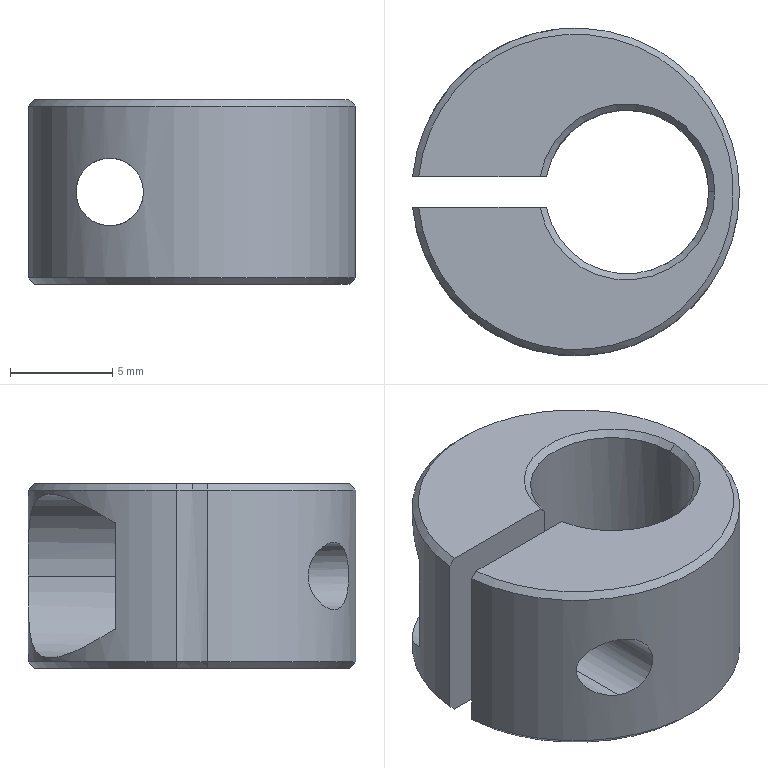Part | NX | features BREP 1 | 1 solid | 19 faces | box 15.965 x 16.002 x 9 mm | volume 1023 mm3 | cylinder 8 | cone 6 | plane 5 | commonest cylinder face diameters 8 x3 3.3 x2 4.5 x2 16 x1
STEP:
#1=CARTESIAN_POINT('',(5.2,0.,-4.5));
#2=VERTEX_POINT('',#1);
#3=CARTESIAN_POINT('',(5.5,0.,-4.2));
#4=VERTEX_POINT('',#3);
#5=CARTESIAN_POINT('',(5.5,0.,-4.2));
#6=DIRECTION('',(0.7071,0.,0.7071));
#7=VECTOR('',#6,1000.);
#8=LINE('',#5,#7);
#9=EDGE_CURVE('',#2,#4,#8,.T.);
#10=ORIENTED_EDGE('',*,*,#9,.F.);
#11=CARTESIAN_POINT('',(-10.163,0.75,-4.5));
#12=VERTEX_POINT('',#11);
#13=CARTESIAN_POINT('',(-2.5,0.,-4.5));
#14=DIRECTION('',(0.,0.,-1.));
#15=DIRECTION('',(1.,0.,0.));
#16=AXIS2_PLACEMENT_3D('',#13,#14,#15);
#17=CIRCLE('',#16,7.7);
#18=EDGE_CURVE('',#12,#2,#17,.T.);
#19=ORIENTED_EDGE('',*,*,#18,.F.);
#20=CARTESIAN_POINT('',(-10.465,0.75,-4.2));
#21=VERTEX_POINT('',#20);
#22=CARTESIAN_POINT('',(-10.465,0.75,-4.2));
#23=CARTESIAN_POINT('',(-10.364,0.75,-4.3));
#24=CARTESIAN_POINT('',(-10.264,0.75,-4.4));
#25=CARTESIAN_POINT('',(-10.163,0.75,-4.5));
#26=B_SPLINE_CURVE_WITH_KNOTS('',3,(#22,#23,#24,#25),.UNSPECIFIED.,.F.,.F.,(4,4),(0.,0.0004252),.UNSPECIFIED.);
#27=EDGE_CURVE('',#21,#12,#26,.T.);
#28=ORIENTED_EDGE('',*,*,#27,.F.);
#29=CARTESIAN_POINT('',(-2.5,0.,-4.2));
#30=DIRECTION('',(0.,0.,1.));
#31=DIRECTION('',(1.,0.,0.));
#32=AXIS2_PLACEMENT_3D('',#29,#30,#31);
#33=CIRCLE('',#32,8.);
#34=EDGE_CURVE('',#4,#21,#33,.T.);
#35=ORIENTED_EDGE('',*,*,#34,.F.);
#36=EDGE_LOOP('',(#10,#19,#28,#35));
#37=FACE_BOUND('',#36,.T.);
#38=CARTESIAN_POINT('',(-2.5,0.,-4.2));
#39=DIRECTION('',(0.,0.,1.));
#40=DIRECTION('',(1.,0.,0.));
#41=AXIS2_PLACEMENT_3D('',#38,#39,#40);
#42=CONICAL_SURFACE('',#41,8.,0.7854);
#43=ADVANCED_FACE('',(#37),#42,.T.);
#44=CARTESIAN_POINT('',(-3.929,-0.75,-4.2));
#45=VERTEX_POINT('',#44);
#46=CARTESIAN_POINT('',(-4.234,-0.75,-4.5));
#47=VERTEX_POINT('',#46);
#48=CARTESIAN_POINT('',(-3.929,-0.75,-4.2));
#49=CARTESIAN_POINT('',(-4.031,-0.75,-4.3));
#50=CARTESIAN_POINT('',(-4.132,-0.75,-4.4));
#51=CARTESIAN_POINT('',(-4.234,-0.75,-4.5));
#52=B_SPLINE_CURVE_WITH_KNOTS('',3,(#48,#49,#50,#51),.UNSPECIFIED.,.F.,.F.,(4,4),(0.,0.0004278),.UNSPECIFIED.);
#53=EDGE_CURVE('',#45,#47,#52,.T.);
#54=ORIENTED_EDGE('',*,*,#53,.F.);
#55=CARTESIAN_POINT('',(-3.929,0.75,-4.2));
#56=VERTEX_POINT('',#55);
#57=CARTESIAN_POINT('',(0.,0.,-4.2));
#58=DIRECTION('',(0.,0.,-1.));
#59=DIRECTION('',(1.,0.,0.));
#60=AXIS2_PLACEMENT_3D('',#57,#58,#59);
#61=CIRCLE('',#60,4.);
#62=EDGE_CURVE('',#56,#45,#61,.T.);
#63=ORIENTED_EDGE('',*,*,#62,.F.);
#64=CARTESIAN_POINT('',(-4.234,0.75,-4.5));
#65=VERTEX_POINT('',#64);
#66=CARTESIAN_POINT('',(-4.234,0.75,-4.5));
#67=CARTESIAN_POINT('',(-4.132,0.75,-4.4));
#68=CARTESIAN_POINT('',(-4.031,0.75,-4.3));
#69=CARTESIAN_POINT('',(-3.929,0.75,-4.2));
#70=B_SPLINE_CURVE_WITH_KNOTS('',3,(#66,#67,#68,#69),.UNSPECIFIED.,.F.,.F.,(4,4),(0.,0.0004278),.UNSPECIFIED.);
#71=EDGE_CURVE('',#65,#56,#70,.T.);
#72=ORIENTED_EDGE('',*,*,#71,.F.);
#73=CARTESIAN_POINT('',(0.,0.,-4.5));
#74=DIRECTION('',(0.,0.,1.));
#75=DIRECTION('',(1.,0.,0.));
#76=AXIS2_PLACEMENT_3D('',#73,#74,#75);
#77=CIRCLE('',#76,4.3);
#78=EDGE_CURVE('',#47,#65,#77,.T.);
#79=ORIENTED_EDGE('',*,*,#78,.F.);
#80=EDGE_LOOP('',(#54,#63,#72,#79));
#81=FACE_BOUND('',#80,.T.);
#82=CARTESIAN_POINT('',(0.,0.,-4.5));
#83=DIRECTION('',(0.,0.,-1.));
#84=DIRECTION('',(-1.,0.,0.));
#85=AXIS2_PLACEMENT_3D('',#82,#83,#84);
#86=CONICAL_SURFACE('',#85,4.3,0.7854);
#87=ADVANCED_FACE('',(#81),#86,.F.);
#88=CARTESIAN_POINT('',(-10.465,-0.75,4.2));
#89=VERTEX_POINT('',#88);
#90=CARTESIAN_POINT('',(-10.163,-0.75,4.5));
#91=VERTEX_POINT('',#90);
#92=CARTESIAN_POINT('',(-10.465,-0.75,4.2));
#93=CARTESIAN_POINT('',(-10.364,-0.75,4.3));
#94=CARTESIAN_POINT('',(-10.264,-0.75,4.4));
#95=CARTESIAN_POINT('',(-10.163,-0.75,4.5));
#96=B_SPLINE_CURVE_WITH_KNOTS('',3,(#92,#93,#94,#95),.UNSPECIFIED.,.F.,.F.,(4,4),(0.,0.0004252),.UNSPECIFIED.);
#97=EDGE_CURVE('',#89,#91,#96,.T.);
#98=ORIENTED_EDGE('',*,*,#97,.F.);
#99=CARTESIAN_POINT('',(-10.465,0.75,4.2));
#100=VERTEX_POINT('',#99);
#101=CARTESIAN_POINT('',(-2.5,0.,4.2));
#102=DIRECTION('',(0.,0.,-1.));
#103=DIRECTION('',(1.,0.,0.));
#104=AXIS2_PLACEMENT_3D('',#101,#102,#103);
#105=CIRCLE('',#104,8.);
#106=EDGE_CURVE('',#100,#89,#105,.T.);
#107=ORIENTED_EDGE('',*,*,#106,.F.);
#108=CARTESIAN_POINT('',(-10.163,0.75,4.5));
#109=VERTEX_POINT('',#108);
#110=CARTESIAN_POINT('',(-10.163,0.75,4.5));
#111=CARTESIAN_POINT('',(-10.264,0.75,4.4));
#112=CARTESIAN_POINT('',(-10.364,0.75,4.3));
#113=CARTESIAN_POINT('',(-10.465,0.75,4.2));
#114=B_SPLINE_CURVE_WITH_KNOTS('',3,(#110,#111,#112,#113),.UNSPECIFIED.,.F.,.F.,(4,4),(0.,0.0004252),.UNSPECIFIED.);
#115=EDGE_CURVE('',#109,#100,#114,.T.);
#116=ORIENTED_EDGE('',*,*,#115,.F.);
#117=CARTESIAN_POINT('',(-2.5,0.,4.5));
#118=DIRECTION('',(0.,0.,1.));
#119=DIRECTION('',(1.,0.,0.));
#120=AXIS2_PLACEMENT_3D('',#117,#118,#119);
#121=CIRCLE('',#120,7.7);
#122=EDGE_CURVE('',#91,#109,#121,.T.);
#123=ORIENTED_EDGE('',*,*,#122,.F.);
#124=EDGE_LOOP('',(#98,#107,#116,#123));
#125=FACE_BOUND('',#124,.T.);
#126=CARTESIAN_POINT('',(-2.5,0.,4.5));
#127=DIRECTION('',(0.,0.,-1.));
#128=DIRECTION('',(-1.,0.,0.));
#129=AXIS2_PLACEMENT_3D('',#126,#127,#128);
#130=CONICAL_SURFACE('',#129,7.7,0.7854);
#131=ADVANCED_FACE('',(#125),#130,.T.);
#132=CARTESIAN_POINT('',(4.,0.,4.2));
#133=VERTEX_POINT('',#132);
#134=CARTESIAN_POINT('',(4.3,0.,4.5));
#135=VERTEX_POINT('',#134);
#136=CARTESIAN_POINT('',(4.,0.,4.2));
#137=DIRECTION('',(0.7071,0.,0.7071));
#138=VECTOR('',#137,1000.);
#139=LINE('',#136,#138);
#140=EDGE_CURVE('',#133,#135,#139,.T.);
#141=ORIENTED_EDGE('',*,*,#140,.F.);
#142=CARTESIAN_POINT('',(-3.929,-0.75,4.2));
#143=VERTEX_POINT('',#142);
#144=CARTESIAN_POINT('',(0.,0.,4.2));
#145=DIRECTION('',(0.,0.,1.));
#146=DIRECTION('',(1.,0.,0.));
#147=AXIS2_PLACEMENT_3D('',#144,#145,#146);
#148=CIRCLE('',#147,4.);
#149=EDGE_CURVE('',#143,#133,#148,.T.);
#150=ORIENTED_EDGE('',*,*,#149,.F.);
#151=CARTESIAN_POINT('',(-4.234,-0.75,4.5));
#152=VERTEX_POINT('',#151);
#153=CARTESIAN_POINT('',(-4.234,-0.75,4.5));
#154=CARTESIAN_POINT('',(-4.132,-0.75,4.4));
#155=CARTESIAN_POINT('',(-4.031,-0.75,4.3));
#156=CARTESIAN_POINT('',(-3.929,-0.75,4.2));
#157=B_SPLINE_CURVE_WITH_KNOTS('',3,(#153,#154,#155,#156),.UNSPECIFIED.,.F.,.F.,(4,4),(0.,0.0004278),.UNSPECIFIED.);
#158=EDGE_CURVE('',#152,#143,#157,.T.);
#159=ORIENTED_EDGE('',*,*,#158,.F.);
#160=CARTESIAN_POINT('',(0.,0.,4.5));
#161=DIRECTION('',(0.,0.,-1.));
#162=DIRECTION('',(1.,0.,0.));
#163=AXIS2_PLACEMENT_3D('',#160,#161,#162);
#164=CIRCLE('',#163,4.3);
#165=EDGE_CURVE('',#135,#152,#164,.T.);
#166=ORIENTED_EDGE('',*,*,#165,.F.);
#167=EDGE_LOOP('',(#141,#150,#159,#166));
#168=FACE_BOUND('',#167,.T.);
#169=CARTESIAN_POINT('',(0.,0.,4.2));
#170=DIRECTION('',(0.,0.,1.));
#171=DIRECTION('',(1.,0.,0.));
#172=AXIS2_PLACEMENT_3D('',#169,#170,#171);
#173=CONICAL_SURFACE('',#172,4.,0.7854);
#174=ADVANCED_FACE('',(#168),#173,.F.);
#175=CARTESIAN_POINT('',(-6.5,-0.75,-1.65));
#176=VERTEX_POINT('',#175);
#177=CARTESIAN_POINT('',(-6.5,-6.928,-1.65));
#178=VERTEX_POINT('',#177);
#179=CARTESIAN_POINT('',(-6.5,-0.75,-1.65));
#180=DIRECTION('',(0.,1.,0.));
#181=VECTOR('',#180,1000.);
#182=LINE('',#179,#181);
#183=EDGE_CURVE('',#176,#178,#182,.F.);
#184=ORIENTED_EDGE('',*,*,#183,.T.);
#185=CARTESIAN_POINT('',(-6.5,-6.928,1.65));
#186=VERTEX_POINT('',#185);
#187=CARTESIAN_POINT('',(-6.5,-6.928,-1.65));
#188=CARTESIAN_POINT('',(-6.079,-7.171,-1.65));
#189=CARTESIAN_POINT('',(-5.272,-7.527,-1.352));
#190=CARTESIAN_POINT('',(-4.638,-7.707,0.003778));
#191=CARTESIAN_POINT('',(-5.276,-7.526,1.354));
#192=CARTESIAN_POINT('',(-6.08,-7.171,1.65));
#193=CARTESIAN_POINT('',(-6.5,-6.928,1.65));
#194=B_SPLINE_CURVE_WITH_KNOTS('',3,(#187,#188,#189,#190,#191,#192,#193),.UNSPECIFIED.,.F.,.F.,(4,1,1,1,4),(0.,0.25,0.5,0.75,1.),.UNSPECIFIED.);
#195=EDGE_CURVE('',#186,#178,#194,.F.);
#196=ORIENTED_EDGE('',*,*,#195,.F.);
#197=CARTESIAN_POINT('',(-6.5,-0.75,1.65));
#198=VERTEX_POINT('',#197);
#199=CARTESIAN_POINT('',(-6.5,-0.75,1.65));
#200=DIRECTION('',(0.,1.,0.));
#201=VECTOR('',#200,1000.);
#202=LINE('',#199,#201);
#203=EDGE_CURVE('',#198,#186,#202,.F.);
#204=ORIENTED_EDGE('',*,*,#203,.F.);
#205=CARTESIAN_POINT('',(-6.5,-0.75,0.));
#206=DIRECTION('',(0.,1.,0.));
#207=DIRECTION('',(0.,0.,1.));
#208=AXIS2_PLACEMENT_3D('',#205,#206,#207);
#209=CIRCLE('',#208,1.65);
#210=EDGE_CURVE('',#198,#176,#209,.T.);
#211=ORIENTED_EDGE('',*,*,#210,.T.);
#212=EDGE_LOOP('',(#184,#196,#204,#211));
#213=FACE_BOUND('',#212,.T.);
#214=CARTESIAN_POINT('',(-6.5,-0.75,0.));
#215=DIRECTION('',(0.,1.,0.));
#216=DIRECTION('',(0.,0.,1.));
#217=AXIS2_PLACEMENT_3D('',#214,#215,#216);
#218=CYLINDRICAL_SURFACE('',#217,1.65);
#219=ADVANCED_FACE('',(#213),#218,.F.);
#220=CARTESIAN_POINT('',(-4.25,0.75,0.));
#221=VERTEX_POINT('',#220);
#222=CARTESIAN_POINT('',(-4.25,3.75,0.));
#223=VERTEX_POINT('',#222);
#224=CARTESIAN_POINT('',(-4.25,-0.25,0.));
#225=DIRECTION('',(0.,1.,0.));
#226=VECTOR('',#225,1000.);
#227=LINE('',#224,#226);
#228=EDGE_CURVE('',#221,#223,#227,.T.);
#229=ORIENTED_EDGE('',*,*,#228,.F.);
#230=CARTESIAN_POINT('',(-8.75,0.75,0.));
#231=VERTEX_POINT('',#230);
#232=CARTESIAN_POINT('',(-6.5,0.75,0.));
#233=DIRECTION('',(0.,1.,0.));
#234=DIRECTION('',(-1.,0.,0.));
#235=AXIS2_PLACEMENT_3D('',#232,#233,#234);
#236=CIRCLE('',#235,2.25);
#237=EDGE_CURVE('',#231,#221,#236,.T.);
#238=ORIENTED_EDGE('',*,*,#237,.F.);
#239=CARTESIAN_POINT('',(-8.75,3.75,0.));
#240=VERTEX_POINT('',#239);
#241=CARTESIAN_POINT('',(-8.75,-0.25,0.));
#242=DIRECTION('',(0.,1.,0.));
#243=VECTOR('',#242,1000.);
#244=LINE('',#241,#243);
#245=EDGE_CURVE('',#231,#240,#244,.T.);
#246=ORIENTED_EDGE('',*,*,#245,.T.);
#247=CARTESIAN_POINT('',(-6.5,3.75,0.));
#248=DIRECTION('',(0.,1.,0.));
#249=DIRECTION('',(-1.,0.,0.));
#250=AXIS2_PLACEMENT_3D('',#247,#248,#249);
#251=CIRCLE('',#250,2.25);
#252=EDGE_CURVE('',#240,#223,#251,.T.);
#253=ORIENTED_EDGE('',*,*,#252,.T.);
#254=EDGE_LOOP('',(#229,#238,#246,#253));
#255=FACE_BOUND('',#254,.T.);
#256=CARTESIAN_POINT('',(-6.5,-0.25,0.));
#257=DIRECTION('',(0.,1.,0.));
#258=DIRECTION('',(-1.,0.,0.));
#259=AXIS2_PLACEMENT_3D('',#256,#257,#258);
#260=CYLINDRICAL_SURFACE('',#259,2.25);
#261=ADVANCED_FACE('',(#255),#260,.F.);
#262=CARTESIAN_POINT('',(-9.567,3.75,-2.568));
#263=VERTEX_POINT('',#262);
#264=CARTESIAN_POINT('',(-2.5,3.75,0.));
#265=VERTEX_POINT('',#264);
#266=CARTESIAN_POINT('',(-6.5,3.75,0.));
#267=DIRECTION('',(0.,-1.,0.));
#268=DIRECTION('',(1.,0.,0.));
#269=AXIS2_PLACEMENT_3D('',#266,#267,#268);
#270=CIRCLE('',#269,4.);
#271=EDGE_CURVE('',#263,#265,#270,.T.);
#272=ORIENTED_EDGE('',*,*,#271,.F.);
#273=CARTESIAN_POINT('',(-9.567,3.75,2.568));
#274=VERTEX_POINT('',#273);
#275=CARTESIAN_POINT('',(-9.567,3.75,4.5));
#276=DIRECTION('',(0.,0.,-1.));
#277=VECTOR('',#276,1000.);
#278=LINE('',#275,#277);
#279=EDGE_CURVE('',#274,#263,#278,.T.);
#280=ORIENTED_EDGE('',*,*,#279,.F.);
#281=CARTESIAN_POINT('',(-6.5,3.75,0.));
#282=DIRECTION('',(0.,-1.,0.));
#283=DIRECTION('',(1.,0.,0.));
#284=AXIS2_PLACEMENT_3D('',#281,#282,#283);
#285=CIRCLE('',#284,4.);
#286=EDGE_CURVE('',#265,#274,#285,.T.);
#287=ORIENTED_EDGE('',*,*,#286,.F.);
#288=EDGE_LOOP('',(#272,#280,#287));
#289=FACE_BOUND('',#288,.T.);
#290=ORIENTED_EDGE('',*,*,#252,.F.);
#291=CARTESIAN_POINT('',(-6.5,3.75,0.));
#292=DIRECTION('',(0.,1.,0.));
#293=DIRECTION('',(-1.,0.,0.));
#294=AXIS2_PLACEMENT_3D('',#291,#292,#293);
#295=CIRCLE('',#294,2.25);
#296=EDGE_CURVE('',#223,#240,#295,.T.);
#297=ORIENTED_EDGE('',*,*,#296,.F.);
#298=EDGE_LOOP('',(#290,#297));
#299=FACE_BOUND('',#298,.T.);
#300=CARTESIAN_POINT('',(-6.5,3.75,0.));
#301=DIRECTION('',(0.,-1.,0.));
#302=DIRECTION('',(1.,0.,0.));
#303=AXIS2_PLACEMENT_3D('',#300,#301,#302);
#304=PLANE('',#303);
#305=ADVANCED_FACE('',(#289,#299),#304,.F.);
#306=CARTESIAN_POINT('',(-2.5,8.,0.));
#307=VERTEX_POINT('',#306);
#308=CARTESIAN_POINT('',(-2.5,11.75,0.));
#309=DIRECTION('',(0.,-1.,0.));
#310=VECTOR('',#309,1000.);
#311=LINE('',#308,#310);
#312=EDGE_CURVE('',#307,#265,#311,.T.);
#313=ORIENTED_EDGE('',*,*,#312,.F.);
#314=CARTESIAN_POINT('',(-2.5,8.,0.));
#315=CARTESIAN_POINT('',(-2.5,8.,-0.3501));
#316=CARTESIAN_POINT('',(-2.562,8.,-0.7752));
#317=CARTESIAN_POINT('',(-2.683,7.998,-1.2));
#318=CARTESIAN_POINT('',(-2.72,7.997,-1.322));
#319=CARTESIAN_POINT('',(-2.902,7.99,-1.769));
#320=CARTESIAN_POINT('',(-3.137,7.975,-2.181));
#321=CARTESIAN_POINT('',(-3.407,7.953,-2.569));
#322=CARTESIAN_POINT('',(-3.972,7.869,-3.129));
#323=CARTESIAN_POINT('',(-4.669,7.716,-3.599));
#324=CARTESIAN_POINT('',(-5.759,7.356,-4.011));
#325=CARTESIAN_POINT('',(-6.811,6.763,-4.016));
#326=CARTESIAN_POINT('',(-7.508,6.252,-3.885));
#327=CARTESIAN_POINT('',(-8.069,5.756,-3.691));
#328=CARTESIAN_POINT('',(-8.447,5.36,-3.503));
#329=CARTESIAN_POINT('',(-8.992,4.71,-3.159));
#330=CARTESIAN_POINT('',(-9.351,4.156,-2.826));
#331=CARTESIAN_POINT('',(-9.567,3.75,-2.568));
#332=B_SPLINE_CURVE_WITH_KNOTS('',3,(#314,#315,#316,#317,#318,#319,#320,#321,#322,#323,#324,#325,#326,#327,#328,#329,#330,#331),.UNSPECIFIED.,.F.,.F.,(4,1,1,1,1,1,1,1,1,1,1,1,1,1,1,4),(0.,0.0625,0.09375,0.125,0.1562,0.1875,0.25,0.3125,0.375,0.5,0.625,0.6875,0.75,0.8125,0.875,1.),.UNSPECIFIED.);
#333=EDGE_CURVE('',#263,#307,#332,.F.);
#334=ORIENTED_EDGE('',*,*,#333,.F.);
#335=ORIENTED_EDGE('',*,*,#271,.T.);
#336=EDGE_LOOP('',(#313,#334,#335));
#337=FACE_BOUND('',#336,.T.);
#338=CARTESIAN_POINT('',(-6.5,11.75,0.));
#339=DIRECTION('',(0.,-1.,0.));
#340=DIRECTION('',(1.,0.,0.));
#341=AXIS2_PLACEMENT_3D('',#338,#339,#340);
#342=CYLINDRICAL_SURFACE('',#341,4.);
#343=ADVANCED_FACE('',(#337),#342,.F.);
#344=CARTESIAN_POINT('',(-13.003,-0.75,4.5));
#345=DIRECTION('',(1.,0.,0.));
#346=VECTOR('',#345,1000.);
#347=LINE('',#344,#346);
#348=EDGE_CURVE('',#91,#152,#347,.T.);
#349=ORIENTED_EDGE('',*,*,#348,.T.);
#350=ORIENTED_EDGE('',*,*,#158,.T.);
#351=CARTESIAN_POINT('',(-3.929,-0.75,4.5));
#352=DIRECTION('',(0.,0.,-1.));
#353=VECTOR('',#352,1000.);
#354=LINE('',#351,#353);
#355=EDGE_CURVE('',#143,#45,#354,.T.);
#356=ORIENTED_EDGE('',*,*,#355,.T.);
#357=ORIENTED_EDGE('',*,*,#53,.T.);
#358=CARTESIAN_POINT('',(-10.163,-0.75,-4.5));
#359=VERTEX_POINT('',#358);
#360=CARTESIAN_POINT('',(-13.003,-0.75,-4.5));
#361=DIRECTION('',(1.,0.,0.));
#362=VECTOR('',#361,1000.);
#363=LINE('',#360,#362);
#364=EDGE_CURVE('',#359,#47,#363,.T.);
#365=ORIENTED_EDGE('',*,*,#364,.F.);
#366=CARTESIAN_POINT('',(-10.465,-0.75,-4.2));
#367=VERTEX_POINT('',#366);
#368=CARTESIAN_POINT('',(-10.163,-0.75,-4.5));
#369=CARTESIAN_POINT('',(-10.264,-0.75,-4.4));
#370=CARTESIAN_POINT('',(-10.364,-0.75,-4.3));
#371=CARTESIAN_POINT('',(-10.465,-0.75,-4.2));
#372=B_SPLINE_CURVE_WITH_KNOTS('',3,(#368,#369,#370,#371),.UNSPECIFIED.,.F.,.F.,(4,4),(0.,0.0004252),.UNSPECIFIED.);
#373=EDGE_CURVE('',#359,#367,#372,.T.);
#374=ORIENTED_EDGE('',*,*,#373,.T.);
#375=CARTESIAN_POINT('',(-10.465,-0.75,4.5));
#376=DIRECTION('',(0.,0.,-1.));
#377=VECTOR('',#376,1000.);
#378=LINE('',#375,#377);
#379=EDGE_CURVE('',#89,#367,#378,.T.);
#380=ORIENTED_EDGE('',*,*,#379,.F.);
#381=ORIENTED_EDGE('',*,*,#97,.T.);
#382=EDGE_LOOP('',(#349,#350,#356,#357,#365,#374,#380,#381));
#383=FACE_BOUND('',#382,.T.);
#384=ORIENTED_EDGE('',*,*,#210,.F.);
#385=CARTESIAN_POINT('',(-6.5,-0.75,0.));
#386=DIRECTION('',(0.,1.,0.));
#387=DIRECTION('',(0.,0.,1.));
#388=AXIS2_PLACEMENT_3D('',#385,#386,#387);
#389=CIRCLE('',#388,1.65);
#390=EDGE_CURVE('',#176,#198,#389,.T.);
#391=ORIENTED_EDGE('',*,*,#390,.F.);
#392=EDGE_LOOP('',(#384,#391));
#393=FACE_BOUND('',#392,.T.);
#394=CARTESIAN_POINT('',(-13.003,-0.75,-4.5));
#395=DIRECTION('',(0.,-1.,0.));
#396=DIRECTION('',(1.,0.,0.));
#397=AXIS2_PLACEMENT_3D('',#394,#395,#396);
#398=PLANE('',#397);
#399=ADVANCED_FACE('',(#383,#393),#398,.F.);
#400=CARTESIAN_POINT('',(-3.929,0.75,4.2));
#401=VERTEX_POINT('',#400);
#402=CARTESIAN_POINT('',(-3.929,0.75,4.5));
#403=DIRECTION('',(0.,0.,1.));
#404=VECTOR('',#403,1000.);
#405=LINE('',#402,#404);
#406=EDGE_CURVE('',#56,#401,#405,.T.);
#407=ORIENTED_EDGE('',*,*,#406,.T.);
#408=CARTESIAN_POINT('',(-4.234,0.75,4.5));
#409=VERTEX_POINT('',#408);
#410=CARTESIAN_POINT('',(-3.929,0.75,4.2));
#411=CARTESIAN_POINT('',(-4.031,0.75,4.3));
#412=CARTESIAN_POINT('',(-4.132,0.75,4.4));
#413=CARTESIAN_POINT('',(-4.234,0.75,4.5));
#414=B_SPLINE_CURVE_WITH_KNOTS('',3,(#410,#411,#412,#413),.UNSPECIFIED.,.F.,.F.,(4,4),(0.,0.0004278),.UNSPECIFIED.);
#415=EDGE_CURVE('',#401,#409,#414,.T.);
#416=ORIENTED_EDGE('',*,*,#415,.T.);
#417=CARTESIAN_POINT('',(-13.003,0.75,4.5));
#418=DIRECTION('',(-1.,0.,0.));
#419=VECTOR('',#418,1000.);
#420=LINE('',#417,#419);
#421=EDGE_CURVE('',#409,#109,#420,.T.);
#422=ORIENTED_EDGE('',*,*,#421,.T.);
#423=ORIENTED_EDGE('',*,*,#115,.T.);
#424=CARTESIAN_POINT('',(-10.465,0.75,4.5));
#425=DIRECTION('',(0.,0.,1.));
#426=VECTOR('',#425,1000.);
#427=LINE('',#424,#426);
#428=EDGE_CURVE('',#21,#100,#427,.T.);
#429=ORIENTED_EDGE('',*,*,#428,.F.);
#430=ORIENTED_EDGE('',*,*,#27,.T.);
#431=CARTESIAN_POINT('',(-13.003,0.75,-4.5));
#432=DIRECTION('',(-1.,0.,0.));
#433=VECTOR('',#432,1000.);
#434=LINE('',#431,#433);
#435=EDGE_CURVE('',#65,#12,#434,.T.);
#436=ORIENTED_EDGE('',*,*,#435,.F.);
#437=ORIENTED_EDGE('',*,*,#71,.T.);
#438=EDGE_LOOP('',(#407,#416,#422,#423,#429,#430,#436,#437));
#439=FACE_BOUND('',#438,.T.);
#440=ORIENTED_EDGE('',*,*,#237,.T.);
#441=CARTESIAN_POINT('',(-6.5,0.75,0.));
#442=DIRECTION('',(0.,1.,0.));
#443=DIRECTION('',(-1.,0.,0.));
#444=AXIS2_PLACEMENT_3D('',#441,#442,#443);
#445=CIRCLE('',#444,2.25);
#446=EDGE_CURVE('',#221,#231,#445,.T.);
#447=ORIENTED_EDGE('',*,*,#446,.T.);
#448=EDGE_LOOP('',(#440,#447));
#449=FACE_BOUND('',#448,.T.);
#450=CARTESIAN_POINT('',(-13.003,0.75,-4.5));
#451=DIRECTION('',(0.,1.,0.));
#452=DIRECTION('',(-1.,0.,0.));
#453=AXIS2_PLACEMENT_3D('',#450,#451,#452);
#454=PLANE('',#453);
#455=ADVANCED_FACE('',(#439,#449),#454,.F.);
#456=ORIENTED_EDGE('',*,*,#355,.F.);
#457=ORIENTED_EDGE('',*,*,#149,.T.);
#458=CARTESIAN_POINT('',(0.,0.,4.2));
#459=DIRECTION('',(0.,0.,1.));
#460=DIRECTION('',(1.,0.,0.));
#461=AXIS2_PLACEMENT_3D('',#458,#459,#460);
#462=CIRCLE('',#461,4.);
#463=EDGE_CURVE('',#133,#401,#462,.T.);
#464=ORIENTED_EDGE('',*,*,#463,.T.);
#465=ORIENTED_EDGE('',*,*,#406,.F.);
#466=ORIENTED_EDGE('',*,*,#62,.T.);
#467=EDGE_LOOP('',(#456,#457,#464,#465,#466));
#468=FACE_BOUND('',#467,.T.);
#469=CARTESIAN_POINT('',(0.,0.,4.5));
#470=DIRECTION('',(0.,0.,-1.));
#471=DIRECTION('',(-1.,0.,0.));
#472=AXIS2_PLACEMENT_3D('',#469,#470,#471);
#473=CYLINDRICAL_SURFACE('',#472,4.);
#474=ADVANCED_FACE('',(#468),#473,.F.);
#475=ORIENTED_EDGE('',*,*,#428,.T.);
#476=ORIENTED_EDGE('',*,*,#106,.T.);
#477=ORIENTED_EDGE('',*,*,#379,.T.);
#478=CARTESIAN_POINT('',(-2.5,0.,-4.2));
#479=DIRECTION('',(0.,0.,1.));
#480=DIRECTION('',(1.,0.,0.));
#481=AXIS2_PLACEMENT_3D('',#478,#479,#480);
#482=CIRCLE('',#481,8.);
#483=EDGE_CURVE('',#367,#4,#482,.T.);
#484=ORIENTED_EDGE('',*,*,#483,.T.);
#485=ORIENTED_EDGE('',*,*,#34,.T.);
#486=EDGE_LOOP('',(#475,#476,#477,#484,#485));
#487=FACE_BOUND('',#486,.T.);
#488=ORIENTED_EDGE('',*,*,#279,.T.);
#489=ORIENTED_EDGE('',*,*,#333,.T.);
#490=CARTESIAN_POINT('',(-2.5,8.,0.));
#491=CARTESIAN_POINT('',(-2.5,8.,0.9356));
#492=CARTESIAN_POINT('',(-3.019,8.024,2.332));
#493=CARTESIAN_POINT('',(-4.461,7.792,3.537));
#494=CARTESIAN_POINT('',(-5.773,7.341,4.));
#495=CARTESIAN_POINT('',(-6.706,6.829,4.024));
#496=CARTESIAN_POINT('',(-7.469,6.286,3.898));
#497=CARTESIAN_POINT('',(-8.063,5.763,3.695));
#498=CARTESIAN_POINT('',(-8.468,5.34,3.494));
#499=CARTESIAN_POINT('',(-9.059,4.619,3.107));
#500=CARTESIAN_POINT('',(-9.362,4.136,2.813));
#501=CARTESIAN_POINT('',(-9.567,3.75,2.568));
#502=B_SPLINE_CURVE_WITH_KNOTS('',3,(#490,#491,#492,#493,#494,#495,#496,#497,#498,#499,#500,#501),.UNSPECIFIED.,.F.,.F.,(4,1,1,1,1,1,1,1,1,4),(0.,0.25,0.375,0.5,0.625,0.6875,0.75,0.8125,0.875,1.),.UNSPECIFIED.);
#503=EDGE_CURVE('',#307,#274,#502,.T.);
#504=ORIENTED_EDGE('',*,*,#503,.T.);
#505=EDGE_LOOP('',(#488,#489,#504));
#506=FACE_BOUND('',#505,.T.);
#507=ORIENTED_EDGE('',*,*,#195,.T.);
#508=CARTESIAN_POINT('',(-6.5,-6.928,-1.65));
#509=CARTESIAN_POINT('',(-6.917,-6.687,-1.65));
#510=CARTESIAN_POINT('',(-7.512,-6.258,-1.414));
#511=CARTESIAN_POINT('',(-8.034,-5.781,-0.7276));
#512=CARTESIAN_POINT('',(-8.208,-5.605,-0.0009844));
#513=CARTESIAN_POINT('',(-8.035,-5.78,0.7251));
#514=CARTESIAN_POINT('',(-7.512,-6.259,1.416));
#515=CARTESIAN_POINT('',(-6.917,-6.687,1.65));
#516=CARTESIAN_POINT('',(-6.5,-6.928,1.65));
#517=B_SPLINE_CURVE_WITH_KNOTS('',3,(#508,#509,#510,#511,#512,#513,#514,#515,#516),.UNSPECIFIED.,.F.,.F.,(4,1,1,1,1,1,4),(0.,0.25,0.375,0.5,0.625,0.75,1.),.UNSPECIFIED.);
#518=EDGE_CURVE('',#178,#186,#517,.T.);
#519=ORIENTED_EDGE('',*,*,#518,.T.);
#520=EDGE_LOOP('',(#507,#519));
#521=FACE_BOUND('',#520,.T.);
#522=CARTESIAN_POINT('',(-2.5,0.,4.5));
#523=DIRECTION('',(0.,0.,-1.));
#524=DIRECTION('',(-1.,0.,0.));
#525=AXIS2_PLACEMENT_3D('',#522,#523,#524);
#526=CYLINDRICAL_SURFACE('',#525,8.);
#527=ADVANCED_FACE('',(#487,#506,#521),#526,.T.);
#528=ORIENTED_EDGE('',*,*,#364,.T.);
#529=ORIENTED_EDGE('',*,*,#78,.T.);
#530=ORIENTED_EDGE('',*,*,#435,.T.);
#531=ORIENTED_EDGE('',*,*,#18,.T.);
#532=CARTESIAN_POINT('',(-2.5,0.,-4.5));
#533=DIRECTION('',(0.,0.,-1.));
#534=DIRECTION('',(1.,0.,0.));
#535=AXIS2_PLACEMENT_3D('',#532,#533,#534);
#536=CIRCLE('',#535,7.7);
#537=EDGE_CURVE('',#2,#359,#536,.T.);
#538=ORIENTED_EDGE('',*,*,#537,.T.);
#539=EDGE_LOOP('',(#528,#529,#530,#531,#538));
#540=FACE_BOUND('',#539,.T.);
#541=CARTESIAN_POINT('',(-2.5,0.,-4.5));
#542=DIRECTION('',(0.,0.,1.));
#543=DIRECTION('',(1.,0.,0.));
#544=AXIS2_PLACEMENT_3D('',#541,#542,#543);
#545=PLANE('',#544);
#546=ADVANCED_FACE('',(#540),#545,.F.);
#547=ORIENTED_EDGE('',*,*,#421,.F.);
#548=CARTESIAN_POINT('',(0.,0.,4.5));
#549=DIRECTION('',(0.,0.,-1.));
#550=DIRECTION('',(1.,0.,0.));
#551=AXIS2_PLACEMENT_3D('',#548,#549,#550);
#552=CIRCLE('',#551,4.3);
#553=EDGE_CURVE('',#409,#135,#552,.T.);
#554=ORIENTED_EDGE('',*,*,#553,.T.);
#555=ORIENTED_EDGE('',*,*,#165,.T.);
#556=ORIENTED_EDGE('',*,*,#348,.F.);
#557=ORIENTED_EDGE('',*,*,#122,.T.);
#558=EDGE_LOOP('',(#547,#554,#555,#556,#557));
#559=FACE_BOUND('',#558,.T.);
#560=CARTESIAN_POINT('',(-2.5,0.,4.5));
#561=DIRECTION('',(0.,0.,1.));
#562=DIRECTION('',(1.,0.,0.));
#563=AXIS2_PLACEMENT_3D('',#560,#561,#562);
#564=PLANE('',#563);
#565=ADVANCED_FACE('',(#559),#564,.T.);
#566=ORIENTED_EDGE('',*,*,#503,.F.);
#567=ORIENTED_EDGE('',*,*,#312,.T.);
#568=ORIENTED_EDGE('',*,*,#286,.T.);
#569=EDGE_LOOP('',(#566,#567,#568));
#570=FACE_BOUND('',#569,.T.);
#571=CARTESIAN_POINT('',(-6.5,11.75,0.));
#572=DIRECTION('',(0.,-1.,0.));
#573=DIRECTION('',(1.,0.,0.));
#574=AXIS2_PLACEMENT_3D('',#571,#572,#573);
#575=CYLINDRICAL_SURFACE('',#574,4.);
#576=ADVANCED_FACE('',(#570),#575,.F.);
#577=ORIENTED_EDGE('',*,*,#446,.F.);
#578=ORIENTED_EDGE('',*,*,#228,.T.);
#579=ORIENTED_EDGE('',*,*,#296,.T.);
#580=ORIENTED_EDGE('',*,*,#245,.F.);
#581=EDGE_LOOP('',(#577,#578,#579,#580));
#582=FACE_BOUND('',#581,.T.);
#583=CARTESIAN_POINT('',(-6.5,-0.25,0.));
#584=DIRECTION('',(0.,1.,0.));
#585=DIRECTION('',(-1.,0.,0.));
#586=AXIS2_PLACEMENT_3D('',#583,#584,#585);
#587=CYLINDRICAL_SURFACE('',#586,2.25);
#588=ADVANCED_FACE('',(#582),#587,.F.);
#589=ORIENTED_EDGE('',*,*,#518,.F.);
#590=ORIENTED_EDGE('',*,*,#183,.F.);
#591=ORIENTED_EDGE('',*,*,#390,.T.);
#592=ORIENTED_EDGE('',*,*,#203,.T.);
#593=EDGE_LOOP('',(#589,#590,#591,#592));
#594=FACE_BOUND('',#593,.T.);
#595=CARTESIAN_POINT('',(-6.5,-0.75,0.));
#596=DIRECTION('',(0.,1.,0.));
#597=DIRECTION('',(0.,0.,1.));
#598=AXIS2_PLACEMENT_3D('',#595,#596,#597);
#599=CYLINDRICAL_SURFACE('',#598,1.65);
#600=ADVANCED_FACE('',(#594),#599,.F.);
#601=ORIENTED_EDGE('',*,*,#463,.F.);
#602=ORIENTED_EDGE('',*,*,#140,.T.);
#603=ORIENTED_EDGE('',*,*,#553,.F.);
#604=ORIENTED_EDGE('',*,*,#415,.F.);
#605=EDGE_LOOP('',(#601,#602,#603,#604));
#606=FACE_BOUND('',#605,.T.);
#607=CARTESIAN_POINT('',(0.,0.,4.2));
#608=DIRECTION('',(0.,0.,1.));
#609=DIRECTION('',(1.,0.,0.));
#610=AXIS2_PLACEMENT_3D('',#607,#608,#609);
#611=CONICAL_SURFACE('',#610,4.,0.7854);
#612=ADVANCED_FACE('',(#606),#611,.F.);
#613=ORIENTED_EDGE('',*,*,#537,.F.);
#614=ORIENTED_EDGE('',*,*,#9,.T.);
#615=ORIENTED_EDGE('',*,*,#483,.F.);
#616=ORIENTED_EDGE('',*,*,#373,.F.);
#617=EDGE_LOOP('',(#613,#614,#615,#616));
#618=FACE_BOUND('',#617,.T.);
#619=CARTESIAN_POINT('',(-2.5,0.,-4.2));
#620=DIRECTION('',(0.,0.,1.));
#621=DIRECTION('',(1.,0.,0.));
#622=AXIS2_PLACEMENT_3D('',#619,#620,#621);
#623=CONICAL_SURFACE('',#622,8.,0.7854);
#624=ADVANCED_FACE('',(#618),#623,.T.);
#625=CLOSED_SHELL('',(#43,#87,#131,#174,#219,#261,#305,#343,#399,#455,#474,#527,#546,#565,#576,#588,#600,#612,#624));
#626=MANIFOLD_SOLID_BREP('',#625);
#627=(LENGTH_UNIT()NAMED_UNIT(*)SI_UNIT(.MILLI.,.METRE.));
#628=UNCERTAINTY_MEASURE_WITH_UNIT(LENGTH_MEASURE(0.0508),#627,'','');
#629=(NAMED_UNIT(*)PLANE_ANGLE_UNIT()SI_UNIT($,.RADIAN.));
#630=(NAMED_UNIT(*)SI_UNIT($,.STERADIAN.)SOLID_ANGLE_UNIT());
#631=(GEOMETRIC_REPRESENTATION_CONTEXT(3)GLOBAL_UNCERTAINTY_ASSIGNED_CONTEXT((#628))GLOBAL_UNIT_ASSIGNED_CONTEXT((#627,#629,#630))REPRESENTATION_CONTEXT('',''));
#632=ADVANCED_BREP_SHAPE_REPRESENTATION('',(#626),#631);